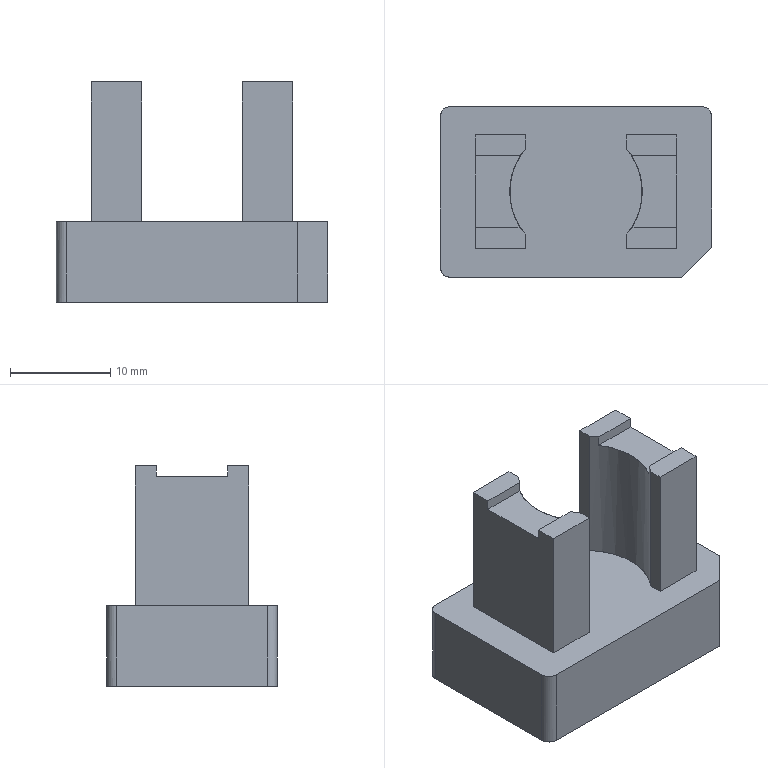NC program | PowerMill | posted with a generic post | part box 27 x 17 x 21.929 mm
Lines 1 to 1024 of 116051:
%
O0001
N104 ( POWERMILL CB  : 2026004.0)
N105 ( POST VER      : 2026.0.0.5161)
N106 ( OPTION FILE   : FANUC)
N107 ( OUTPUT WORKPLANE : WORLD)
N108 (  )
N109 ( TOOL LIST )
N110 (---------------------------------------)
N111 ( NO. | ID        | DIA.| TIP RAD|LENGTH)
N112 (---------------------------------------)
N113 (    1|D10C_1_1_1 |10.0 |  0.0   |77.36 )
N114 (    2|D4C_1_1    | 4.0 |  0.0   |69.12 )
N115 (    3|D10_1_1_1  |10.0 |  0.0   |77.08 )
N116 (   14|D4_1_1     | 4.0 |  0.0   |69.08 )
N117 (   13|TEXT_D4_1_1| 4.0 |  0.3   | 69.2 )
N118 (---------------------------------------)
N119 (  )
N120 ( NUMBER OF TOOLPATHS: 10.0 )
N121 ( ESTIMATED PROGRAM DURATION: 0 HOURS 13 MIN 49 SEC)
N122 (  )
N123 G00 G21 G80 G40 G17
N124 G90
N125 G54
N126 G53 Z0.0
N127 (---------------)
N128 ( START TOOLPATH : 精公开粗01-扫面平行-D10C )
N129 (---------------)
N130 ( TOOL NO.    :1 )
N131 ( TOOL TYPE   : ENDMILL)
N132 ( TOOL ID     : D10C_1_1_1)
N133 ( TOOL DIA    : 10.0 LENGTH 77.36)
N134 T1
N135 M6
N136 S8000 M03
N137 G00 G90 X0.0 Y0.0
N138 G43 Z10.2 H1
N139
N140 G05 P10000 R4
N141 X21.28 Y11.28
N142 Z1.129
N143 G01 Z-0.071 F6000.0
N144 X16.28 F10000.0
N145 X-16.28
N146 Y5.64
N147 X16.28
N148 Y0.0
N149 X-16.28
N150 Y-5.64
N151 X16.28
N152 Y-11.28
N153 X-16.28
N154 X-21.28
N155 G00 Z10.2
N156 G05 P0
N157 (---------------)
N158 ( END TOOLPATH : 精公开粗01-扫面平行-D10C )
N159 (---------------)
N160 ( START TOOLPATH : 精公开粗01-外形偏置-D10C )
N161 (---------------)
N162 G00 X0.0 Y0.0 Z9.879
N163 G05 P10000 R4
N164 X-2.5948 Y-18.709
N165 Z0.6842
N166 G01 Z-0.5158 F6000.0
N167 Y-18.1815 F10000.0
N168 G03 X-7.3423 Y-13.434 I-4.7475 J0.0
N169 G01 X-16.827
N170 G02 X-17.827 Y-12.434 I0.0 J1.0
N171 G01 Y12.434
N172 G02 X-16.827 Y13.434 I1.0 J0.0
N173 G01 X16.827
N174 G02 X17.827 Y12.434 I0.0 J-1.0
N175 G01 Y-12.434
N176 G02 X16.827 Y-13.434 I-1.0 J0.0
N177 G01 X-7.3423
N178 X-7.3476 Y-10.929
N179 X-10.0545 Y-10.9347
N180 X-10.828 Y-10.8766
N181 X-11.6014 Y-10.7008
N182 X-12.3748 Y-10.3941
N183 X-13.1483 Y-9.9283
N184 X-13.885 Y-9.2811
N185 X-14.4903 Y-8.5077
N186 X-14.6951 Y-8.1603
N187 X-14.9006 Y-7.7343
N188 X-15.1633 Y-6.9608
N189 X-15.3005 Y-6.1874
N190 X-15.3274 Y-5.414
N191 X-15.306 Y-3.0937
N192 X-15.181 Y-2.3203
N193 X-14.9384 Y-1.5469
N194 X-14.6951 Y-1.0402
N195 X-14.5393 Y-0.7734
N196 X-14.1877 Y-0.3054
N197 G03 X-14.2024 Y0.314 I-0.3997 J0.3003
N198 G01 X-14.2643 Y0.3886
N199 X-14.6951 Y1.0607
N200 X-14.9264 Y1.5469
N201 X-15.1809 Y2.3203
N202 X-15.306 Y3.0937
N203 X-15.3274 Y5.414
N204 X-15.3005 Y6.1874
N205 X-15.1633 Y6.9608
N206 X-14.9006 Y7.7343
N207 X-14.6951 Y8.1602
N208 X-14.4903 Y8.5077
N209 X-13.9217 Y9.242
N210 X-13.1483 Y9.9283
N211 X-12.3748 Y10.3941
N212 X-11.6014 Y10.7008
N213 X-10.828 Y10.8766
N214 X-10.0545 Y10.9347
N215 X-4.6406 Y10.9233
N216 X-3.9302 Y10.828
N217 X-3.0937 Y10.5837
N218 X-2.3203 Y10.2121
N219 X-2.0675 Y10.0545
N220 X-1.5469 Y9.6607
N221 X-1.1488 Y9.2811
N222 X-0.7734 Y8.8373
N223 X-0.5436 Y8.5077
N224 X-0.4435 Y8.3167
N225 G03 X0.4411 Y8.3145 I0.4429 J0.2321
N226 G01 X0.5436 Y8.5077
N227 X0.7734 Y8.8373
N228 X1.1488 Y9.2811
N229 X1.5469 Y9.6607
N230 X2.0675 Y10.0545
N231 X2.3203 Y10.2121
N232 X3.0937 Y10.5837
N233 X3.8671 Y10.8147
N234 X4.6406 Y10.9233
N235 X10.0545 Y10.9347
N236 X10.828 Y10.8766
N237 X11.6014 Y10.7008
N238 X12.3748 Y10.3941
N239 X13.1483 Y9.9283
N240 X13.885 Y9.2811
N241 X14.4903 Y8.5077
N242 X14.6951 Y8.1602
N243 X14.9006 Y7.7343
N244 X15.1633 Y6.9608
N245 X15.3005 Y6.1874
N246 X15.3274 Y5.414
N247 X15.306 Y3.0937
N248 X15.1809 Y2.3203
N249 X14.9264 Y1.5469
N250 X14.6951 Y1.0607
N251 X14.2643 Y0.3887
N252 X14.2027 Y0.3144
N253 G03 X14.1874 Y-0.3044 I0.3849 J-0.3191
N254 G01 X14.5385 Y-0.7734
N255 X14.6951 Y-1.0402
N256 X14.9384 Y-1.5469
N257 X15.181 Y-2.3203
N258 X15.306 Y-3.0937
N259 X15.3274 Y-5.414
N260 X15.3005 Y-6.1874
N261 X15.1633 Y-6.9608
N262 X14.9006 Y-7.7343
N263 X14.6951 Y-8.1603
N264 X14.4903 Y-8.5077
N265 X13.9217 Y-9.242
N266 X13.1483 Y-9.9283
N267 X12.3748 Y-10.3941
N268 X11.6014 Y-10.7008
N269 X11.1036 Y-10.828
N270 X10.828 Y-10.8766
N271 X10.0545 Y-10.9347
N272 X4.6406 Y-10.9233
N273 X3.9302 Y-10.828
N274 X3.0937 Y-10.5837
N275 X2.3203 Y-10.2121
N276 X2.0675 Y-10.0545
N277 X1.5469 Y-9.6606
N278 X1.1488 Y-9.2811
N279 X0.7734 Y-8.8373
N280 X0.5436 Y-8.5077
N281 X0.4417 Y-8.3156
N282 G03 X-0.4417 I-0.4417 J-0.2344
N283 G01 X-0.5436 Y-8.5077
N284 X-0.7734 Y-8.8373
N285 X-1.1488 Y-9.2811
N286 X-1.5469 Y-9.6606
N287 X-2.0675 Y-10.0545
N288 X-2.3203 Y-10.2121
N289 X-3.0937 Y-10.5837
N290 X-3.8671 Y-10.8147
N291 X-4.6406 Y-10.9233
N292 X-7.3476 Y-10.929
N293 X-7.3423 Y-13.434
N294 G00 Z3.2894
N295 G01 X-2.5948 Y-18.709
N296 G00 Z0.2893
N297 G01 Z-0.9107 F6000.0
N298 Y-18.1815 F10000.0
N299 G03 X-7.3423 Y-13.434 I-4.7475 J0.0
N300 G01 X-16.827
N301 G02 X-17.827 Y-12.434 I0.0 J1.0
N302 G01 Y12.434
N303 G02 X-16.827 Y13.434 I1.0 J0.0
N304 G01 X-7.3423
N305 X-7.3476 Y10.929
N306 X-4.6406 Y10.9233
N307 X-3.9302 Y10.828
N308 X-3.0937 Y10.5837
N309 X-2.3203 Y10.2121
N310 X-2.0675 Y10.0545
N311 X-1.5469 Y9.6607
N312 X-1.1488 Y9.2811
N313 X-0.7734 Y8.8373
N314 X-0.5436 Y8.5077
N315 X-0.4435 Y8.3167
N316 G03 X0.4411 Y8.3145 I0.4429 J0.2321
N317 G01 X0.5436 Y8.5077
N318 X0.7734 Y8.8373
N319 X1.1488 Y9.2811
N320 X1.5469 Y9.6607
N321 X2.0675 Y10.0545
N322 X2.3203 Y10.2121
N323 X3.0937 Y10.5837
N324 X3.8671 Y10.8147
N325 X4.6406 Y10.9233
N326 X10.0545 Y10.9347
N327 X10.828 Y10.8766
N328 X11.6014 Y10.7008
N329 X12.3748 Y10.3941
N330 X13.1483 Y9.9283
N331 X13.885 Y9.2811
N332 X14.4903 Y8.5077
N333 X14.6951 Y8.1602
N334 X14.9006 Y7.7343
N335 X15.1633 Y6.9608
N336 X15.3005 Y6.1874
N337 X15.3274 Y5.414
N338 X15.3084 Y3.0937
N339 X15.1859 Y2.3203
N340 X14.9314 Y1.5469
N341 X14.8685 Y1.4253
N342 X14.6951 Y1.0607
N343 X14.6168 Y0.9386
N344 X14.5314 Y0.7734
N345 X14.264 Y0.3883
N346 X14.2041 Y0.316
N347 G03 X14.1897 Y-0.3041 I0.3849 J-0.3192
N348 G01 X14.5435 Y-0.7734
N349 X14.5806 Y-0.8452
N350 X14.6951 Y-1.0402
N351 X14.8717 Y-1.4081
N352 X14.9434 Y-1.5469
N353 X15.186 Y-2.3203
N354 X15.3084 Y-3.0937
N355 X15.3274 Y-5.414
N356 X15.3005 Y-6.1874
N357 X15.1633 Y-6.9608
N358 X14.9006 Y-7.7343
N359 X14.6951 Y-8.1603
N360 X14.4903 Y-8.5077
N361 X13.9217 Y-9.242
N362 X13.1483 Y-9.9283
N363 X12.3748 Y-10.3941
N364 X11.6014 Y-10.7008
N365 X11.1036 Y-10.828
N366 X10.828 Y-10.8766
N367 X10.0545 Y-10.9347
N368 X4.6406 Y-10.9233
N369 X3.9302 Y-10.828
N370 X3.0937 Y-10.5837
N371 X2.3203 Y-10.2121
N372 X2.0675 Y-10.0545
N373 X1.5469 Y-9.6606
N374 X1.1488 Y-9.2811
N375 X0.7734 Y-8.8373
N376 X0.5436 Y-8.5077
N377 X0.4417 Y-8.3156
N378 G03 X-0.4417 I-0.4417 J-0.2344
N379 G01 X-0.5436 Y-8.5077
N380 X-0.7734 Y-8.8373
N381 X-1.1488 Y-9.2811
N382 X-1.5469 Y-9.6606
N383 X-2.0675 Y-10.0545
N384 X-2.3203 Y-10.2121
N385 X-3.0937 Y-10.5837
N386 X-3.8671 Y-10.8147
N387 X-4.6406 Y-10.9233
N388 X-10.0545 Y-10.9347
N389 X-10.828 Y-10.8766
N390 X-11.6014 Y-10.7008
N391 X-12.3748 Y-10.3941
N392 X-13.1483 Y-9.9283
N393 X-13.885 Y-9.2811
N394 X-14.4903 Y-8.5077
N395 X-14.6951 Y-8.1603
N396 X-14.9006 Y-7.7343
N397 X-15.1633 Y-6.9608
N398 X-15.3005 Y-6.1874
N399 X-15.3274 Y-5.414
N400 X-15.3084 Y-3.0937
N401 X-15.186 Y-2.3203
N402 X-14.9434 Y-1.5469
N403 X-14.8705 Y-1.4056
N404 X-14.6951 Y-1.0402
N405 X-14.5802 Y-0.8435
N406 X-14.544 Y-0.7734
N407 X-14.1882 Y-0.3036
N408 X-14.1291 Y-0.203
N409 X-14.0949 Y-0.0915
N410 G03 X-14.2024 Y0.314 I-0.4925 J0.0864
N411 G01 X-14.2642 Y0.3887
N412 X-14.3509 Y0.5239
N413 X-14.5326 Y0.7734
N414 X-14.6217 Y0.9462
N415 X-14.6951 Y1.0607
N416 X-14.8662 Y1.4205
N417 X-14.9314 Y1.5469
N418 X-15.1859 Y2.3203
N419 X-15.3084 Y3.0937
N420 X-15.3274 Y5.414
N421 X-15.3005 Y6.1874
N422 X-15.1633 Y6.9608
N423 X-14.9006 Y7.7343
N424 X-14.6951 Y8.1602
N425 X-14.4903 Y8.5077
N426 X-13.9217 Y9.242
N427 X-13.1483 Y9.9283
N428 X-12.3748 Y10.3941
N429 X-11.6014 Y10.7008
N430 X-10.828 Y10.8766
N431 X-10.0545 Y10.9347
N432 X-7.3476 Y10.929
N433 X-7.3423 Y13.434
N434 X16.827
N435 G02 X17.827 Y12.434 I0.0 J-1.0
N436 G01 Y-12.434
N437 G02 X16.827 Y-13.434 I-1.0 J0.0
N438 G01 X-7.3423
N439 G00 Z2.8945
N440 G01 X-2.5948 Y-18.709
N441 G00 Z-0.1055
N442 G01 Z-1.3055 F6000.0
N443 Y-18.1815 F10000.0
N444 G03 X-7.3423 Y-13.434 I-4.7475 J0.0
N445 G01 X-16.827
N446 G02 X-17.827 Y-12.434 I0.0 J1.0
N447 G01 Y12.434
N448 G02 X-16.827 Y13.434 I1.0 J0.0
N449 G01 X16.827
N450 G02 X17.827 Y12.434 I0.0 J-1.0
N451 G01 Y0.0
N452 X15.3275
N453 Y-5.414
N454 X15.3005 Y-6.1874
N455 X15.1633 Y-6.9608
N456 X14.9006 Y-7.7343
N457 X14.6951 Y-8.1603
N458 X14.4903 Y-8.5077
N459 X13.9217 Y-9.242
N460 X13.1483 Y-9.9283
N461 X12.3748 Y-10.3941
N462 X11.6014 Y-10.7008
N463 X11.1036 Y-10.828
N464 X10.828 Y-10.8767
N465 X10.0545 Y-10.9347
N466 X4.6406 Y-10.9233
N467 X3.9302 Y-10.828
N468 X3.0937 Y-10.5837
N469 X2.3203 Y-10.2121
N470 X2.0675 Y-10.0545
N471 X1.5469 Y-9.6606
N472 X1.1488 Y-9.2811
N473 X0.7734 Y-8.8373
N474 X0.5436 Y-8.5077
N475 X0.4417 Y-8.3156
N476 G03 X-0.4417 I-0.4417 J-0.2344
N477 G01 X-0.5436 Y-8.5077
N478 X-0.7734 Y-8.8373
N479 X-1.1488 Y-9.2811
N480 X-1.5469 Y-9.6606
N481 X-2.0675 Y-10.0545
N482 X-2.3203 Y-10.2121
N483 X-3.0937 Y-10.5837
N484 X-3.8671 Y-10.8147
N485 X-4.6406 Y-10.9233
N486 X-10.0545 Y-10.9347
N487 X-10.828 Y-10.8767
N488 X-11.6014 Y-10.7008
N489 X-12.3748 Y-10.3941
N490 X-13.1483 Y-9.9283
N491 X-13.885 Y-9.2811
N492 X-14.4903 Y-8.5077
N493 X-14.6951 Y-8.1603
N494 X-14.9006 Y-7.7343
N495 X-15.1633 Y-6.9608
N496 X-15.3005 Y-6.1874
N497 X-15.3275 Y-5.414
N498 Y5.414
N499 X-15.3005 Y6.1874
N500 X-15.1633 Y6.9608
N501 X-14.9006 Y7.7343
N502 X-14.6951 Y8.1602
N503 X-14.4903 Y8.5077
N504 X-13.9217 Y9.242
N505 X-13.1483 Y9.9283
N506 X-12.3748 Y10.3941
N507 X-11.6014 Y10.7008
N508 X-10.828 Y10.8767
N509 X-10.0545 Y10.9347
N510 X-4.6406 Y10.9233
N511 X-3.9302 Y10.828
N512 X-3.0937 Y10.5837
N513 X-2.3203 Y10.2121
N514 X-2.0675 Y10.0545
N515 X-1.5469 Y9.6607
N516 X-1.1488 Y9.2811
N517 X-0.7734 Y8.8373
N518 X-0.5436 Y8.5077
N519 X-0.5343 Y8.4898
N520 X-0.4435 Y8.3167
N521 G03 X0.4214 Y8.2805 I0.4429 J0.2321
N522 G01 X0.4314 Y8.297
N523 X0.4408 Y8.3139
N524 X0.5436 Y8.5077
N525 X0.7734 Y8.8373
N526 X1.1488 Y9.2811
N527 X1.5469 Y9.6607
N528 X2.0675 Y10.0545
N529 X2.3203 Y10.2121
N530 X3.0937 Y10.5837
N531 X3.8671 Y10.8147
N532 X4.6406 Y10.9233
N533 X10.0545 Y10.9347
N534 X10.828 Y10.8767
N535 X11.6014 Y10.7008
N536 X12.3748 Y10.3941
N537 X13.1483 Y9.9283
N538 X13.885 Y9.2811
N539 X14.4903 Y8.5077
N540 X14.6951 Y8.1602
N541 X14.9006 Y7.7343
N542 X15.1633 Y6.9608
N543 X15.3005 Y6.1874
N544 X15.3275 Y5.414
N545 Y0.0
N546 X17.827
N547 Y-12.434
N548 G02 X16.827 Y-13.434 I-1.0 J0.0
N549 G01 X-7.3423
N550 G00 Z2.4997
N551 G01 X-2.5948 Y-18.709
N552 G00 Z-0.5003
N553 G01 Z-1.7003 F6000.0
N554 Y-18.1815 F10000.0
N555 G03 X-7.3423 Y-13.434 I-4.7475 J0.0
N556 G01 X-16.827
N557 G02 X-17.827 Y-12.434 I0.0 J1.0
N558 G01 Y12.434
N559 G02 X-16.827 Y13.434 I1.0 J0.0
N560 G01 X16.827
N561 G02 X17.827 Y12.434 I0.0 J-1.0
N562 G01 Y0.0
N563 X15.3275
N564 Y-5.414
N565 X15.3005 Y-6.1874
N566 X15.1633 Y-6.9608
N567 X14.9006 Y-7.7343
N568 X14.6951 Y-8.1603
N569 X14.4903 Y-8.5077
N570 X13.9217 Y-9.242
N571 X13.1483 Y-9.9283
N572 X12.3748 Y-10.3941
N573 X11.6014 Y-10.7009
N574 X11.1036 Y-10.828
N575 X10.828 Y-10.8767
N576 X10.0545 Y-10.9347
N577 X4.6406 Y-10.9233
N578 X3.9302 Y-10.828
N579 X3.0937 Y-10.5837
N580 X2.3203 Y-10.2121
N581 X2.0675 Y-10.0545
N582 X1.5469 Y-9.6606
N583 X1.1488 Y-9.2811
N584 X0.7734 Y-8.8373
N585 X0.5436 Y-8.5077
N586 X0.4417 Y-8.3156
N587 G03 X-0.4417 I-0.4417 J-0.2344
N588 G01 X-0.5436 Y-8.5077
N589 X-0.7734 Y-8.8373
N590 X-1.1488 Y-9.2811
N591 X-1.5469 Y-9.6606
N592 X-2.0675 Y-10.0545
N593 X-2.3203 Y-10.2121
N594 X-3.0937 Y-10.5837
N595 X-3.8671 Y-10.8147
N596 X-4.6406 Y-10.9233
N597 X-10.0545 Y-10.9347
N598 X-10.828 Y-10.8767
N599 X-11.6014 Y-10.7009
N600 X-12.3748 Y-10.3941
N601 X-13.1483 Y-9.9283
N602 X-13.885 Y-9.2811
N603 X-14.4903 Y-8.5077
N604 X-14.6951 Y-8.1603
N605 X-14.9006 Y-7.7343
N606 X-15.1633 Y-6.9608
N607 X-15.3005 Y-6.1874
N608 X-15.3275 Y-5.414
N609 Y5.414
N610 X-15.3005 Y6.1874
N611 X-15.1633 Y6.9608
N612 X-14.9006 Y7.7343
N613 X-14.6951 Y8.1602
N614 X-14.4903 Y8.5077
N615 X-13.9217 Y9.242
N616 X-13.1483 Y9.9283
N617 X-12.3748 Y10.3941
N618 X-11.6014 Y10.7009
N619 X-10.828 Y10.8767
N620 X-10.0545 Y10.9347
N621 X-4.6406 Y10.9233
N622 X-3.9302 Y10.828
N623 X-3.0937 Y10.5837
N624 X-2.3203 Y10.2121
N625 X-2.0675 Y10.0545
N626 X-1.5469 Y9.6607
N627 X-1.1488 Y9.2811
N628 X-0.7734 Y8.8373
N629 X-0.5436 Y8.5077
N630 X-0.5249 Y8.4719
N631 X-0.4436 Y8.3166
N632 G03 X0.3988 Y8.2478 I0.443 J0.2322
N633 G01 X0.4211 Y8.28
N634 X0.4408 Y8.3139
N635 X0.5436 Y8.5077
N636 X0.7734 Y8.8373
N637 X1.1488 Y9.2811
N638 X1.5469 Y9.6607
N639 X2.0675 Y10.0545
N640 X2.3203 Y10.2121
N641 X3.0937 Y10.5837
N642 X3.8671 Y10.8147
N643 X4.6406 Y10.9233
N644 X10.0545 Y10.9347
N645 X10.828 Y10.8767
N646 X11.6014 Y10.7009
N647 X12.3748 Y10.3941
N648 X13.1483 Y9.9283
N649 X13.885 Y9.2811
N650 X14.4903 Y8.5077
N651 X14.6951 Y8.1602
N652 X14.9006 Y7.7343
N653 X15.1633 Y6.9608
N654 X15.3005 Y6.1874
N655 X15.3275 Y5.414
N656 Y0.0
N657 X17.827
N658 Y-12.434
N659 G02 X16.827 Y-13.434 I-1.0 J0.0
N660 G01 X-7.3423
N661 G00 Z2.1049
N662 G01 X-2.5948 Y-18.709
N663 G00 Z-0.8951
N664 G01 Z-2.0951 F6000.0
N665 Y-18.1815 F10000.0
N666 G03 X-7.3423 Y-13.434 I-4.7475 J0.0
N667 G01 X-16.827
N668 G02 X-17.827 Y-12.434 I0.0 J1.0
N669 G01 Y12.434
N670 G02 X-16.827 Y13.434 I1.0 J0.0
N671 G01 X16.827
N672 G02 X17.827 Y12.434 I0.0 J-1.0
N673 G01 Y0.0
N674 X15.3275
N675 Y-5.414
N676 X15.3005 Y-6.1874
N677 X15.1633 Y-6.9608
N678 X14.9006 Y-7.7343
N679 X14.6951 Y-8.1603
N680 X14.4903 Y-8.5077
N681 X13.9217 Y-9.242
N682 X13.1483 Y-9.9283
N683 X12.3748 Y-10.3941
N684 X11.6014 Y-10.7009
N685 X11.1037 Y-10.828
N686 X10.828 Y-10.8767
N687 X10.0545 Y-10.9347
N688 X4.6406 Y-10.9233
N689 X3.9302 Y-10.828
N690 X3.0937 Y-10.5837
N691 X2.3203 Y-10.2121
N692 X2.0675 Y-10.0545
N693 X1.5469 Y-9.6606
N694 X1.1488 Y-9.2811
N695 X0.7734 Y-8.8373
N696 X0.5436 Y-8.5077
N697 X0.4417 Y-8.3156
N698 G03 X-0.4417 I-0.4417 J-0.2344
N699 G01 X-0.5436 Y-8.5077
N700 X-0.7734 Y-8.8373
N701 X-1.1488 Y-9.2811
N702 X-1.5469 Y-9.6606
N703 X-2.0675 Y-10.0545
N704 X-2.3203 Y-10.2121
N705 X-3.0937 Y-10.5837
N706 X-3.8671 Y-10.8147
N707 X-4.6406 Y-10.9233
N708 X-10.0545 Y-10.9347
N709 X-10.828 Y-10.8767
N710 X-11.6014 Y-10.7009
N711 X-12.3748 Y-10.3941
N712 X-13.1483 Y-9.9283
N713 X-13.885 Y-9.2811
N714 X-14.4903 Y-8.5077
N715 X-14.6951 Y-8.1603
N716 X-14.9006 Y-7.7343
N717 X-15.1633 Y-6.9608
N718 X-15.3005 Y-6.1874
N719 X-15.3275 Y-5.414
N720 Y5.414
N721 X-15.3005 Y6.1874
N722 X-15.1633 Y6.9608
N723 X-14.9006 Y7.7343
N724 X-14.6951 Y8.1602
N725 X-14.4903 Y8.5077
N726 X-13.9217 Y9.242
N727 X-13.1483 Y9.9283
N728 X-12.3748 Y10.3941
N729 X-11.6014 Y10.7009
N730 X-10.828 Y10.8767
N731 X-10.0545 Y10.9347
N732 X-4.6406 Y10.9233
N733 X-3.9302 Y10.828
N734 X-3.0937 Y10.5837
N735 X-2.3203 Y10.2121
N736 X-2.0675 Y10.0545
N737 X-1.5469 Y9.6607
N738 X-1.1488 Y9.2811
N739 X-0.7734 Y8.8373
N740 X-0.5436 Y8.5077
N741 X-0.5156 Y8.454
N742 X-0.4436 Y8.3166
N743 G03 X0.373 Y8.2163 I0.443 J0.2322
N744 G01 X0.4098 Y8.2631
N745 X0.4408 Y8.3139
N746 X0.5436 Y8.5077
N747 X0.7734 Y8.8373
N748 X1.1488 Y9.2811
N749 X1.5469 Y9.6607
N750 X2.0675 Y10.0545
N751 X2.3203 Y10.2121
N752 X3.0937 Y10.5837
N753 X3.8671 Y10.8147
N754 X4.6406 Y10.9233
N755 X10.0545 Y10.9347
N756 X10.828 Y10.8767
N757 X11.6014 Y10.7009
N758 X12.3748 Y10.3941
N759 X13.1483 Y9.9283
N760 X13.885 Y9.2811
N761 X14.4903 Y8.5077
N762 X14.6951 Y8.1602
N763 X14.9006 Y7.7343
N764 X15.1633 Y6.9608
N765 X15.3005 Y6.1874
N766 X15.3275 Y5.414
N767 Y0.0
N768 X17.827
N769 Y-12.434
N770 G02 X16.827 Y-13.434 I-1.0 J0.0
N771 G01 X-7.3423
N772 G00 Z1.71
N773 G01 X-2.5948 Y-18.709
N774 G00 Z-1.29
N775 G01 Z-2.49 F6000.0
N776 Y-18.1815 F10000.0
N777 G03 X-7.3423 Y-13.434 I-4.7475 J0.0
N778 G01 X-16.827
N779 G02 X-17.827 Y-12.434 I0.0 J1.0
N780 G01 Y12.434
N781 G02 X-16.827 Y13.434 I1.0 J0.0
N782 G01 X16.827
N783 G02 X17.827 Y12.434 I0.0 J-1.0
N784 G01 Y0.0
N785 X15.3275
N786 Y-5.414
N787 X15.3005 Y-6.1874
N788 X15.1633 Y-6.9608
N789 X14.9006 Y-7.7343
N790 X14.6951 Y-8.1603
N791 X14.4903 Y-8.5077
N792 X13.9217 Y-9.242
N793 X13.1483 Y-9.9283
N794 X12.3748 Y-10.3941
N795 X11.6014 Y-10.7009
N796 X11.1037 Y-10.828
N797 X10.828 Y-10.8767
N798 X10.0545 Y-10.9347
N799 X4.6406 Y-10.9233
N800 X3.9302 Y-10.828
N801 X3.0937 Y-10.5837
N802 X2.3203 Y-10.2121
N803 X2.0675 Y-10.0545
N804 X1.5469 Y-9.6606
N805 X1.1488 Y-9.2811
N806 X0.7734 Y-8.8373
N807 X0.5436 Y-8.5077
N808 X0.4417 Y-8.3156
N809 G03 X-0.4417 I-0.4417 J-0.2344
N810 G01 X-0.5436 Y-8.5077
N811 X-0.7734 Y-8.8373
N812 X-1.1488 Y-9.2811
N813 X-1.5469 Y-9.6606
N814 X-2.0675 Y-10.0545
N815 X-2.3203 Y-10.2121
N816 X-3.0937 Y-10.5837
N817 X-3.8671 Y-10.8147
N818 X-4.6406 Y-10.9233
N819 X-10.0545 Y-10.9347
N820 X-10.828 Y-10.8767
N821 X-11.6014 Y-10.7009
N822 X-12.3748 Y-10.3941
N823 X-13.1483 Y-9.9283
N824 X-13.885 Y-9.2811
N825 X-14.4903 Y-8.5077
N826 X-14.6951 Y-8.1603
N827 X-14.9006 Y-7.7343
N828 X-15.1633 Y-6.9608
N829 X-15.3005 Y-6.1874
N830 X-15.3275 Y-5.414
N831 Y5.414
N832 X-15.3005 Y6.1874
N833 X-15.1633 Y6.9608
N834 X-14.9006 Y7.7343
N835 X-14.6951 Y8.1602
N836 X-14.4903 Y8.5077
N837 X-13.9217 Y9.242
N838 X-13.1483 Y9.9283
N839 X-12.3748 Y10.3941
N840 X-11.6014 Y10.7009
N841 X-10.828 Y10.8767
N842 X-10.0545 Y10.9347
N843 X-4.6406 Y10.9233
N844 X-3.9302 Y10.828
N845 X-3.0937 Y10.5837
N846 X-2.3203 Y10.2121
N847 X-2.0675 Y10.0545
N848 X-1.5469 Y9.6607
N849 X-1.1488 Y9.2811
N850 X-0.7734 Y8.8373
N851 X-0.5436 Y8.5077
N852 X-0.5063 Y8.436
N853 X-0.4436 Y8.3166
N854 G03 X0.3438 Y8.1861 I0.443 J0.2322
N855 G01 X0.3974 Y8.2461
N856 X0.4408 Y8.3139
N857 X0.5436 Y8.5077
N858 X0.7734 Y8.8373
N859 X1.1488 Y9.2811
N860 X1.5469 Y9.6607
N861 X2.0675 Y10.0545
N862 X2.3203 Y10.2121
N863 X3.0937 Y10.5837
N864 X3.8671 Y10.8147
N865 X4.6406 Y10.9233
N866 X10.0545 Y10.9347
N867 X10.828 Y10.8767
N868 X11.6014 Y10.7009
N869 X12.3748 Y10.3941
N870 X13.1483 Y9.9283
N871 X13.885 Y9.2811
N872 X14.4903 Y8.5077
N873 X14.6951 Y8.1602
N874 X14.9006 Y7.7343
N875 X15.1633 Y6.9608
N876 X15.3005 Y6.1874
N877 X15.3275 Y5.414
N878 Y0.0
N879 X17.827
N880 Y-12.434
N881 G02 X16.827 Y-13.434 I-1.0 J0.0
N882 G01 X-7.3423
N883 G00 Z1.3152
N884 G01 X-2.5948 Y-18.709
N885 G00 Z-1.6848
N886 G01 Z-2.8848 F6000.0
N887 Y-18.1815 F10000.0
N888 G03 X-7.3423 Y-13.434 I-4.7475 J0.0
N889 G01 X-16.827
N890 G02 X-17.827 Y-12.434 I0.0 J1.0
N891 G01 Y12.434
N892 G02 X-16.827 Y13.434 I1.0 J0.0
N893 G01 X16.827
N894 G02 X17.827 Y12.434 I0.0 J-1.0
N895 G01 Y0.0
N896 X15.3275
N897 Y-5.414
N898 X15.3005 Y-6.1874
N899 X15.1633 Y-6.9608
N900 X14.9006 Y-7.7343
N901 X14.6951 Y-8.1603
N902 X14.4903 Y-8.5077
N903 X13.9217 Y-9.242
N904 X13.1483 Y-9.9283
N905 X12.3748 Y-10.3941
N906 X11.6014 Y-10.7009
N907 X11.1037 Y-10.828
N908 X10.828 Y-10.8767
N909 X10.0545 Y-10.9347
N910 X4.6406 Y-10.9233
N911 X3.9302 Y-10.828
N912 X3.0937 Y-10.5838
N913 X2.3203 Y-10.2121
N914 X2.0675 Y-10.0545
N915 X1.5469 Y-9.6606
N916 X1.1488 Y-9.2811
N917 X0.7734 Y-8.8373
N918 X0.5436 Y-8.5077
N919 X0.4417 Y-8.3156
N920 G03 X-0.4417 I-0.4417 J-0.2344
N921 G01 X-0.5436 Y-8.5077
N922 X-0.7734 Y-8.8373
N923 X-1.1488 Y-9.2811
N924 X-1.5469 Y-9.6606
N925 X-2.0675 Y-10.0545
N926 X-2.3203 Y-10.2121
N927 X-3.0937 Y-10.5838
N928 X-3.8671 Y-10.8147
N929 X-4.6406 Y-10.9233
N930 X-10.0545 Y-10.9347
N931 X-10.828 Y-10.8767
N932 X-11.6014 Y-10.7009
N933 X-12.3748 Y-10.3941
N934 X-13.1483 Y-9.9283
N935 X-13.885 Y-9.2811
N936 X-14.4903 Y-8.5077
N937 X-14.6951 Y-8.1603
N938 X-14.9006 Y-7.7343
N939 X-15.1633 Y-6.9608
N940 X-15.3005 Y-6.1874
N941 X-15.3275 Y-5.414
N942 Y5.414
N943 X-15.3005 Y6.1874
N944 X-15.1633 Y6.9608
N945 X-14.9006 Y7.7343
N946 X-14.6951 Y8.1602
N947 X-14.4903 Y8.5077
N948 X-13.9217 Y9.242
N949 X-13.1483 Y9.9283
N950 X-12.3748 Y10.3941
N951 X-11.6014 Y10.7009
N952 X-10.828 Y10.8767
N953 X-10.0545 Y10.9347
N954 X-4.6406 Y10.9233
N955 X-3.9302 Y10.828
N956 X-3.0937 Y10.5838
N957 X-2.3203 Y10.2121
N958 X-2.0675 Y10.0545
N959 X-1.5469 Y9.6607
N960 X-1.1488 Y9.2811
N961 X-0.7734 Y8.8374
N962 X-0.5436 Y8.5077
N963 X-0.4969 Y8.4181
N964 X-0.4437 Y8.3166
N965 G03 X0.3109 Y8.1574 I0.4431 J0.2322
N966 G01 X0.3839 Y8.229
N967 X0.4408 Y8.3139
N968 X0.5436 Y8.5077
N969 X0.7734 Y8.8374
N970 X1.1488 Y9.2811
N971 X1.5469 Y9.6607
N972 X2.0675 Y10.0545
N973 X2.3203 Y10.2121
N974 X3.0937 Y10.5838
N975 X3.8671 Y10.8147
N976 X4.6406 Y10.9233
N977 X10.0545 Y10.9347
N978 X10.828 Y10.8767
N979 X11.6014 Y10.7009
N980 X12.3748 Y10.3941
N981 X13.1483 Y9.9283
N982 X13.885 Y9.2811
N983 X14.4903 Y8.5077
N984 X14.6951 Y8.1602
N985 X14.9006 Y7.7343
N986 X15.1633 Y6.9608
N987 X15.3005 Y6.1874
N988 X15.3275 Y5.414
N989 Y0.0
N990 X17.827
N991 Y-12.434
N992 G02 X16.827 Y-13.434 I-1.0 J0.0
N993 G01 X-7.3423
N994 G00 Z0.9204
N995 G01 X-2.5948 Y-18.709
N996 G00 Z-2.0796
N997 G01 Z-3.2796 F6000.0
N998 Y-18.1815 F10000.0
N999 G03 X-7.3423 Y-13.434 I-4.7475 J0.0
N1000 G01 X-16.827
N1001 G02 X-17.827 Y-12.434 I0.0 J1.0
N1002 G01 Y12.434
N1003 G02 X-16.827 Y13.434 I1.0 J0.0
N1004 G01 X16.827
N1005 G02 X17.827 Y12.434 I0.0 J-1.0
N1006 G01 Y0.0
N1007 X15.3275
N1008 Y-5.414
N1009 X15.3005 Y-6.1874
N1010 X15.1633 Y-6.9608
N1011 X14.9006 Y-7.7343
N1012 X14.6951 Y-8.1603
N1013 X14.4903 Y-8.5077
N1014 X13.9217 Y-9.2421
N1015 X13.1483 Y-9.9283
N1016 X12.3748 Y-10.3941
N1017 X11.6014 Y-10.7009
N1018 X11.1037 Y-10.828
N1019 X10.828 Y-10.8767
N1020 X10.0545 Y-10.9347
N1021 X4.6406 Y-10.9233
N1022 X3.9302 Y-10.828
N1023 X3.0937 Y-10.5838
N1024 X2.3203 Y-10.2121
N1025 X2.0675 Y-10.0545
N1026 X1.5469 Y-9.6606
N1027 X1.1488 Y-9.2811
N1028 X0.7734 Y-8.8373
N1029 X0.5436 Y-8.5077
N1030 X0.4417 Y-8.3157
N1031 G03 X-0.4417 I-0.4417 J-0.2343
N1032 G01 X-0.5436 Y-8.5077
N1033 X-0.7734 Y-8.8373
N1034 X-1.1488 Y-9.2811
N1035 X-1.5469 Y-9.6606
N1036 X-2.0675 Y-10.0545
N1037 X-2.3203 Y-10.2121
N1038 X-3.0937 Y-10.5838
N1039 X-3.8671 Y-10.8147
N1040 X-4.6406 Y-10.9233
N1041 X-10.0545 Y-10.9347
N1042 X-10.828 Y-10.8767
N1043 X-11.6014 Y-10.7009
N1044 X-12.3748 Y-10.3941
N1045 X-13.1483 Y-9.9283
N1046 X-13.885 Y-9.2811
N1047 X-14.4903 Y-8.5077
N1048 X-14.6951 Y-8.1603
N1049 X-14.9006 Y-7.7343
N1050 X-15.1633 Y-6.9608
N1051 X-15.3005 Y-6.1874
N1052 X-15.3275 Y-5.414
N1053 Y5.414
N1054 X-15.3005 Y6.1874
N1055 X-15.1633 Y6.9608
N1056 X-14.9006 Y7.7343
N1057 X-14.6951 Y8.1602
N1058 X-14.4903 Y8.5077
N1059 X-13.9217 Y9.2421
N1060 X-13.1483 Y9.9283
N1061 X-12.3748 Y10.3941
N1062 X-11.6014 Y10.7009
N1063 X-10.828 Y10.8767
N1064 X-10.0545 Y10.9347
N1065 X-4.6406 Y10.9233
N1066 X-3.9302 Y10.828
N1067 X-3.0937 Y10.5838
N1068 X-2.3203 Y10.2121
N1069 X-2.0675 Y10.0545
N1070 X-1.5469 Y9.6607
N1071 X-1.1488 Y9.2811
N1072 X-0.7734 Y8.8374
N1073 X-0.5436 Y8.5077
N1074 X-0.4876 Y8.4002
N1075 X-0.4437 Y8.3165
N1076 G03 X0.2737 Y8.1304 I0.4431 J0.2323
N1077 G01 X0.3688 Y8.2116
N1078 X0.4408 Y8.3139
N1079 X0.5436 Y8.5077
N1080 X0.7734 Y8.8374
N1081 X1.1488 Y9.2811
N1082 X1.5469 Y9.6607
N1083 X2.0675 Y10.0545
N1084 X2.3203 Y10.2121
N1085 X3.0937 Y10.5838
N1086 X3.8671 Y10.8147
N1087 X4.6406 Y10.9233
N1088 X10.0545 Y10.9347
N1089 X10.828 Y10.8767
N1090 X11.6014 Y10.7009
N1091 X12.3748 Y10.3941
N1092 X13.1483 Y9.9283
N1093 X13.885 Y9.2811
N1094 X14.4903 Y8.5077
N1095 X14.6951 Y8.1602
N1096 X14.9006 Y7.7343
N1097 X15.1633 Y6.9608
N1098 X15.3005 Y6.1874
N1099 X15.3275 Y5.414
N1100 Y0.0
N1101 X17.827
N1102 Y-12.434
N1103 G02 X16.827 Y-13.434 I-1.0 J0.0
N1104 G01 X-7.3423
N1105 G00 Z0.5256
N1106 G01 X-2.5948 Y-18.709
N1107 G00 Z-2.4744
N1108 G01 Z-3.6744 F6000.0
N1109 Y-18.1815 F10000.0
N1110 G03 X-7.3423 Y-13.434 I-4.7475 J0.0
N1111 G01 X-16.827
N1112 G02 X-17.827 Y-12.434 I0.0 J1.0
N1113 G01 Y12.434
N1114 G02 X-16.827 Y13.434 I1.0 J0.0
N1115 G01 X16.827
N1116 G02 X17.827 Y12.434 I0.0 J-1.0
N1117 G01 Y0.0
N1118 X15.3275
N1119 Y-5.414
N1120 X15.3005 Y-6.1874
N1121 X15.1633 Y-6.9608